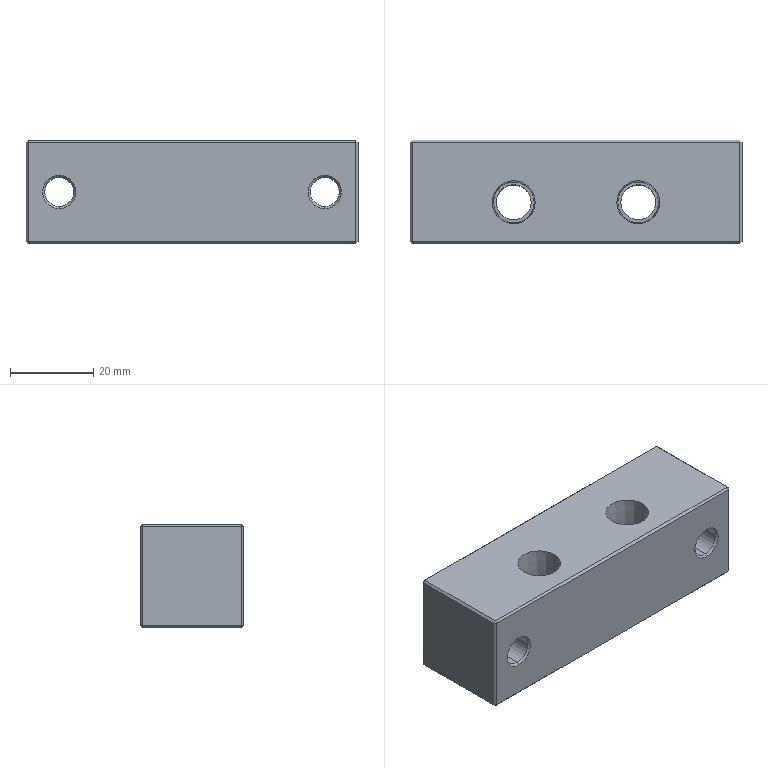Part | STEP file | OP10-161_junction block (G) | 1 solid | 72 faces | box 80 x 25 x 25 mm | volume 42075 mm3 | plane 34 | cone 20 | cylinder 18 | commonest cylinder face diameters 8.433 x10 7 x4 11 x4